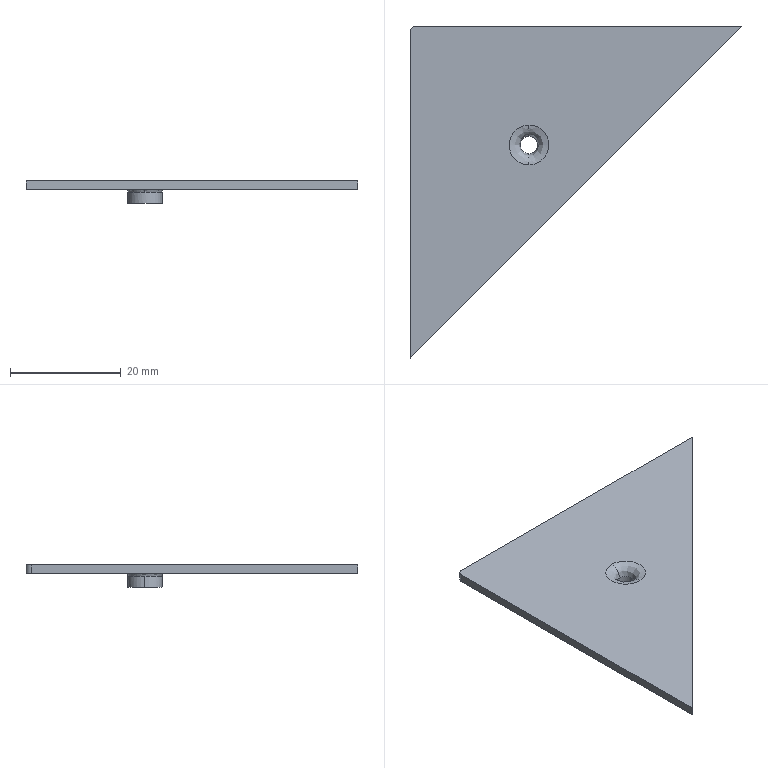Part | STEP file | HESS-408-70-15W-W-9-outer case triangular plate | 1 solid | 15 faces | box 60 x 60 x 4 mm | volume 2733 mm3 | plane 6 | cylinder 5 | spline 4 | commonest cylinder face diameters 3.2 x2 6.2 x2 2 x1